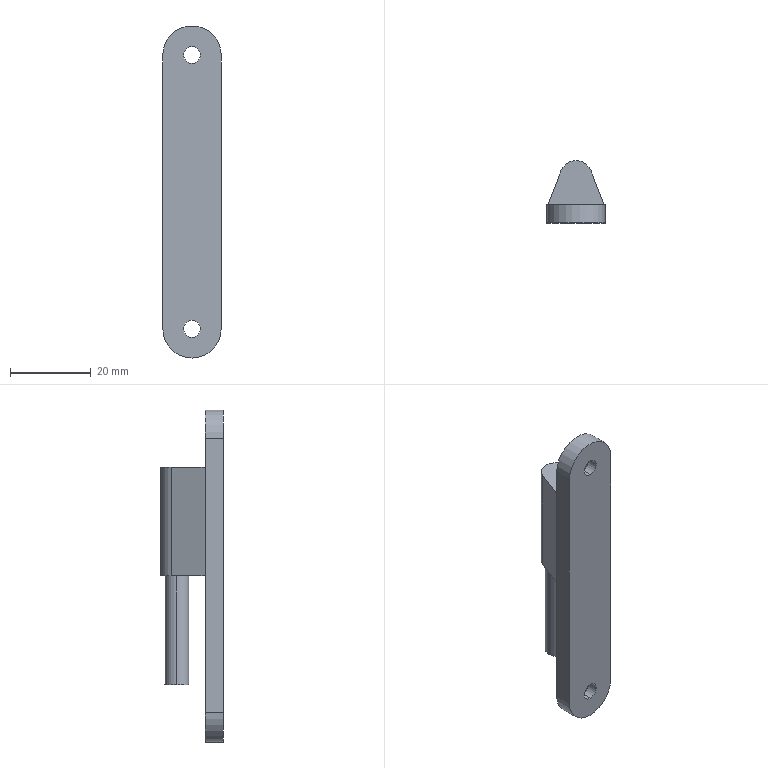Part | SolidWorks | features BaseBody 1 | 1 solid | 23 faces | box 14.5 x 15.5 x 82.5 mm | volume 8558 mm3 | cylinder 10 | plane 9 | cone 4 | commonest cylinder face diameters 4.2 x4 14.5 x3 6 x2 8 x1
STEP:
#1=CARTESIAN_POINT('',(-7.25,-7.,-34.));
#2=VERTEX_POINT('',#1);
#3=CARTESIAN_POINT('',(0.,-7.,-41.25));
#4=VERTEX_POINT('',#3);
#5=CARTESIAN_POINT('',(0.,-7.,-34.));
#6=DIRECTION('',(0.,-1.,0.));
#7=DIRECTION('',(0.,0.,-1.));
#8=AXIS2_PLACEMENT_3D('',#5,#6,#7);
#9=CIRCLE('',#8,7.25);
#10=EDGE_CURVE('',#2,#4,#9,.T.);
#11=ORIENTED_EDGE('',*,*,#10,.T.);
#12=CARTESIAN_POINT('',(0.,-11.5,-41.25));
#13=VERTEX_POINT('',#12);
#14=CARTESIAN_POINT('',(0.,-11.5,-41.25));
#15=DIRECTION('',(0.,-1.,0.));
#16=VECTOR('',#15,1000.);
#17=LINE('',#14,#16);
#18=EDGE_CURVE('',#4,#13,#17,.T.);
#19=ORIENTED_EDGE('',*,*,#18,.T.);
#20=CARTESIAN_POINT('',(-7.25,-11.5,-34.));
#21=VERTEX_POINT('',#20);
#22=CARTESIAN_POINT('',(0.,-11.5,-34.));
#23=DIRECTION('',(0.,1.,0.));
#24=DIRECTION('',(0.,0.,-1.));
#25=AXIS2_PLACEMENT_3D('',#22,#23,#24);
#26=CIRCLE('',#25,7.25);
#27=EDGE_CURVE('',#13,#21,#26,.T.);
#28=ORIENTED_EDGE('',*,*,#27,.T.);
#29=CARTESIAN_POINT('',(-7.25,-11.5,-34.));
#30=DIRECTION('',(0.,-1.,0.));
#31=VECTOR('',#30,1000.);
#32=LINE('',#29,#31);
#33=EDGE_CURVE('',#2,#21,#32,.T.);
#34=ORIENTED_EDGE('',*,*,#33,.F.);
#35=EDGE_LOOP('',(#11,#19,#28,#34));
#36=FACE_OUTER_BOUND('',#35,.T.);
#37=CARTESIAN_POINT('',(0.,-11.5,-34.));
#38=DIRECTION('',(0.,-1.,0.));
#39=DIRECTION('',(0.,0.,-1.));
#40=AXIS2_PLACEMENT_3D('',#37,#38,#39);
#41=CYLINDRICAL_SURFACE('',#40,7.25);
#42=ADVANCED_FACE('',(#36),#41,.T.);
#43=CARTESIAN_POINT('',(0.,-9.,36.1));
#44=VERTEX_POINT('',#43);
#45=CARTESIAN_POINT('',(0.,-9.,31.9));
#46=VERTEX_POINT('',#45);
#47=CARTESIAN_POINT('',(0.,-9.,34.));
#48=DIRECTION('',(0.,-1.,0.));
#49=DIRECTION('',(0.,0.,-1.));
#50=AXIS2_PLACEMENT_3D('',#47,#48,#49);
#51=CIRCLE('',#50,2.1);
#52=EDGE_CURVE('',#44,#46,#51,.T.);
#53=ORIENTED_EDGE('',*,*,#52,.F.);
#54=CARTESIAN_POINT('',(0.,-11.5,36.1));
#55=VERTEX_POINT('',#54);
#56=CARTESIAN_POINT('',(0.,-11.5,36.1));
#57=DIRECTION('',(0.,-1.,0.));
#58=VECTOR('',#57,1000.);
#59=LINE('',#56,#58);
#60=EDGE_CURVE('',#44,#55,#59,.T.);
#61=ORIENTED_EDGE('',*,*,#60,.T.);
#62=CARTESIAN_POINT('',(0.,-11.5,31.9));
#63=VERTEX_POINT('',#62);
#64=CARTESIAN_POINT('',(0.,-11.5,34.));
#65=DIRECTION('',(0.,-1.,0.));
#66=DIRECTION('',(0.,0.,-1.));
#67=AXIS2_PLACEMENT_3D('',#64,#65,#66);
#68=CIRCLE('',#67,2.1);
#69=EDGE_CURVE('',#55,#63,#68,.T.);
#70=ORIENTED_EDGE('',*,*,#69,.T.);
#71=CARTESIAN_POINT('',(0.,-11.5,31.9));
#72=DIRECTION('',(0.,-1.,0.));
#73=VECTOR('',#72,1000.);
#74=LINE('',#71,#73);
#75=EDGE_CURVE('',#46,#63,#74,.T.);
#76=ORIENTED_EDGE('',*,*,#75,.F.);
#77=EDGE_LOOP('',(#53,#61,#70,#76));
#78=FACE_OUTER_BOUND('',#77,.T.);
#79=CARTESIAN_POINT('',(0.,-11.5,34.));
#80=DIRECTION('',(0.,-1.,0.));
#81=DIRECTION('',(0.,0.,-1.));
#82=AXIS2_PLACEMENT_3D('',#79,#80,#81);
#83=CYLINDRICAL_SURFACE('',#82,2.1);
#84=ADVANCED_FACE('',(#78),#83,.F.);
#85=CARTESIAN_POINT('',(0.,-9.,-31.9));
#86=VERTEX_POINT('',#85);
#87=CARTESIAN_POINT('',(0.,-9.,-36.1));
#88=VERTEX_POINT('',#87);
#89=CARTESIAN_POINT('',(0.,-9.,-34.));
#90=DIRECTION('',(0.,-1.,0.));
#91=DIRECTION('',(0.,0.,-1.));
#92=AXIS2_PLACEMENT_3D('',#89,#90,#91);
#93=CIRCLE('',#92,2.1);
#94=EDGE_CURVE('',#86,#88,#93,.T.);
#95=ORIENTED_EDGE('',*,*,#94,.F.);
#96=CARTESIAN_POINT('',(0.,-11.5,-31.9));
#97=VERTEX_POINT('',#96);
#98=CARTESIAN_POINT('',(0.,-11.5,-31.9));
#99=DIRECTION('',(0.,-1.,0.));
#100=VECTOR('',#99,1000.);
#101=LINE('',#98,#100);
#102=EDGE_CURVE('',#86,#97,#101,.T.);
#103=ORIENTED_EDGE('',*,*,#102,.T.);
#104=CARTESIAN_POINT('',(0.,-11.5,-36.1));
#105=VERTEX_POINT('',#104);
#106=CARTESIAN_POINT('',(0.,-11.5,-34.));
#107=DIRECTION('',(0.,-1.,0.));
#108=DIRECTION('',(0.,0.,-1.));
#109=AXIS2_PLACEMENT_3D('',#106,#107,#108);
#110=CIRCLE('',#109,2.1);
#111=EDGE_CURVE('',#97,#105,#110,.T.);
#112=ORIENTED_EDGE('',*,*,#111,.T.);
#113=CARTESIAN_POINT('',(0.,-11.5,-36.1));
#114=DIRECTION('',(0.,-1.,0.));
#115=VECTOR('',#114,1000.);
#116=LINE('',#113,#115);
#117=EDGE_CURVE('',#88,#105,#116,.T.);
#118=ORIENTED_EDGE('',*,*,#117,.F.);
#119=EDGE_LOOP('',(#95,#103,#112,#118));
#120=FACE_OUTER_BOUND('',#119,.T.);
#121=CARTESIAN_POINT('',(0.,-11.5,-34.));
#122=DIRECTION('',(0.,-1.,0.));
#123=DIRECTION('',(0.,0.,-1.));
#124=AXIS2_PLACEMENT_3D('',#121,#122,#123);
#125=CYLINDRICAL_SURFACE('',#124,2.1);
#126=ADVANCED_FACE('',(#120),#125,.F.);
#127=ORIENTED_EDGE('',*,*,#52,.T.);
#128=CARTESIAN_POINT('',(0.,-7.,29.9));
#129=VERTEX_POINT('',#128);
#130=CARTESIAN_POINT('',(0.,-7.,29.9));
#131=DIRECTION('',(0.,0.7071,-0.7071));
#132=VECTOR('',#131,1000.);
#133=LINE('',#130,#132);
#134=EDGE_CURVE('',#46,#129,#133,.T.);
#135=ORIENTED_EDGE('',*,*,#134,.T.);
#136=CARTESIAN_POINT('',(0.,-7.,38.1));
#137=VERTEX_POINT('',#136);
#138=CARTESIAN_POINT('',(0.,-7.,34.));
#139=DIRECTION('',(0.,-1.,0.));
#140=DIRECTION('',(0.,0.,1.));
#141=AXIS2_PLACEMENT_3D('',#138,#139,#140);
#142=CIRCLE('',#141,4.1);
#143=EDGE_CURVE('',#137,#129,#142,.T.);
#144=ORIENTED_EDGE('',*,*,#143,.F.);
#145=CARTESIAN_POINT('',(0.,-7.,38.1));
#146=DIRECTION('',(0.,0.7071,0.7071));
#147=VECTOR('',#146,1000.);
#148=LINE('',#145,#147);
#149=EDGE_CURVE('',#44,#137,#148,.T.);
#150=ORIENTED_EDGE('',*,*,#149,.F.);
#151=EDGE_LOOP('',(#127,#135,#144,#150));
#152=FACE_OUTER_BOUND('',#151,.T.);
#153=CARTESIAN_POINT('',(0.,-7.,34.));
#154=DIRECTION('',(0.,1.,0.));
#155=DIRECTION('',(0.,0.,1.));
#156=AXIS2_PLACEMENT_3D('',#153,#154,#155);
#157=CONICAL_SURFACE('',#156,4.1,0.7854);
#158=ADVANCED_FACE('',(#152),#157,.F.);
#159=ORIENTED_EDGE('',*,*,#94,.T.);
#160=CARTESIAN_POINT('',(0.,-7.,-38.1));
#161=VERTEX_POINT('',#160);
#162=CARTESIAN_POINT('',(0.,-7.,-38.1));
#163=DIRECTION('',(0.,0.7071,-0.7071));
#164=VECTOR('',#163,1000.);
#165=LINE('',#162,#164);
#166=EDGE_CURVE('',#88,#161,#165,.T.);
#167=ORIENTED_EDGE('',*,*,#166,.T.);
#168=CARTESIAN_POINT('',(0.,-7.,-29.9));
#169=VERTEX_POINT('',#168);
#170=CARTESIAN_POINT('',(0.,-7.,-34.));
#171=DIRECTION('',(0.,-1.,0.));
#172=DIRECTION('',(0.,0.,1.));
#173=AXIS2_PLACEMENT_3D('',#170,#171,#172);
#174=CIRCLE('',#173,4.1);
#175=EDGE_CURVE('',#169,#161,#174,.T.);
#176=ORIENTED_EDGE('',*,*,#175,.F.);
#177=CARTESIAN_POINT('',(0.,-7.,-29.9));
#178=DIRECTION('',(0.,0.7071,0.7071));
#179=VECTOR('',#178,1000.);
#180=LINE('',#177,#179);
#181=EDGE_CURVE('',#86,#169,#180,.T.);
#182=ORIENTED_EDGE('',*,*,#181,.F.);
#183=EDGE_LOOP('',(#159,#167,#176,#182));
#184=FACE_OUTER_BOUND('',#183,.T.);
#185=CARTESIAN_POINT('',(0.,-7.,-34.));
#186=DIRECTION('',(0.,1.,0.));
#187=DIRECTION('',(0.,0.,1.));
#188=AXIS2_PLACEMENT_3D('',#185,#186,#187);
#189=CONICAL_SURFACE('',#188,4.1,0.7854);
#190=ADVANCED_FACE('',(#184),#189,.F.);
#191=CARTESIAN_POINT('',(3.,0.,-27.));
#192=VERTEX_POINT('',#191);
#193=CARTESIAN_POINT('',(-3.,0.,-27.));
#194=VERTEX_POINT('',#193);
#195=CARTESIAN_POINT('',(0.,0.,-27.));
#196=DIRECTION('',(0.,0.,1.));
#197=DIRECTION('',(1.,0.,0.));
#198=AXIS2_PLACEMENT_3D('',#195,#196,#197);
#199=CIRCLE('',#198,3.);
#200=EDGE_CURVE('',#192,#194,#199,.T.);
#201=ORIENTED_EDGE('',*,*,#200,.T.);
#202=CARTESIAN_POINT('',(-3.,0.,0.));
#203=VERTEX_POINT('',#202);
#204=CARTESIAN_POINT('',(-3.,0.,27.));
#205=DIRECTION('',(0.,0.,1.));
#206=VECTOR('',#205,1000.);
#207=LINE('',#204,#206);
#208=EDGE_CURVE('',#194,#203,#207,.T.);
#209=ORIENTED_EDGE('',*,*,#208,.T.);
#210=CARTESIAN_POINT('',(3.,0.,0.));
#211=VERTEX_POINT('',#210);
#212=CARTESIAN_POINT('',(0.,0.,0.));
#213=DIRECTION('',(0.,0.,-1.));
#214=DIRECTION('',(1.,0.,0.));
#215=AXIS2_PLACEMENT_3D('',#212,#213,#214);
#216=CIRCLE('',#215,3.);
#217=EDGE_CURVE('',#203,#211,#216,.T.);
#218=ORIENTED_EDGE('',*,*,#217,.T.);
#219=CARTESIAN_POINT('',(3.,0.,27.));
#220=DIRECTION('',(0.,0.,1.));
#221=VECTOR('',#220,1000.);
#222=LINE('',#219,#221);
#223=EDGE_CURVE('',#192,#211,#222,.T.);
#224=ORIENTED_EDGE('',*,*,#223,.F.);
#225=EDGE_LOOP('',(#201,#209,#218,#224));
#226=FACE_OUTER_BOUND('',#225,.T.);
#227=CARTESIAN_POINT('',(0.,0.,27.));
#228=DIRECTION('',(0.,0.,1.));
#229=DIRECTION('',(1.,0.,0.));
#230=AXIS2_PLACEMENT_3D('',#227,#228,#229);
#231=CYLINDRICAL_SURFACE('',#230,3.);
#232=ADVANCED_FACE('',(#226),#231,.T.);
#233=CARTESIAN_POINT('',(7.25,-11.5,-34.));
#234=VERTEX_POINT('',#233);
#235=CARTESIAN_POINT('',(0.,-11.5,-34.));
#236=DIRECTION('',(0.,1.,0.));
#237=DIRECTION('',(0.,0.,-1.));
#238=AXIS2_PLACEMENT_3D('',#235,#236,#237);
#239=CIRCLE('',#238,7.25);
#240=EDGE_CURVE('',#234,#13,#239,.T.);
#241=ORIENTED_EDGE('',*,*,#240,.F.);
#242=CARTESIAN_POINT('',(7.25,-11.5,34.));
#243=VERTEX_POINT('',#242);
#244=CARTESIAN_POINT('',(7.25,-11.5,34.));
#245=DIRECTION('',(0.,0.,-1.));
#246=VECTOR('',#245,1000.);
#247=LINE('',#244,#246);
#248=EDGE_CURVE('',#243,#234,#247,.T.);
#249=ORIENTED_EDGE('',*,*,#248,.F.);
#250=CARTESIAN_POINT('',(-7.25,-11.5,34.));
#251=VERTEX_POINT('',#250);
#252=CARTESIAN_POINT('',(0.,-11.5,34.));
#253=DIRECTION('',(0.,1.,0.));
#254=DIRECTION('',(0.,0.,-1.));
#255=AXIS2_PLACEMENT_3D('',#252,#253,#254);
#256=CIRCLE('',#255,7.25);
#257=EDGE_CURVE('',#251,#243,#256,.T.);
#258=ORIENTED_EDGE('',*,*,#257,.F.);
#259=CARTESIAN_POINT('',(-7.25,-11.5,34.));
#260=DIRECTION('',(0.,0.,1.));
#261=VECTOR('',#260,1000.);
#262=LINE('',#259,#261);
#263=EDGE_CURVE('',#21,#251,#262,.T.);
#264=ORIENTED_EDGE('',*,*,#263,.F.);
#265=ORIENTED_EDGE('',*,*,#27,.F.);
#266=EDGE_LOOP('',(#241,#249,#258,#264,#265));
#267=FACE_OUTER_BOUND('',#266,.T.);
#268=CARTESIAN_POINT('',(0.,-11.5,34.));
#269=DIRECTION('',(0.,-1.,0.));
#270=DIRECTION('',(0.,0.,-1.));
#271=AXIS2_PLACEMENT_3D('',#268,#269,#270);
#272=CIRCLE('',#271,2.1);
#273=EDGE_CURVE('',#63,#55,#272,.T.);
#274=ORIENTED_EDGE('',*,*,#273,.F.);
#275=ORIENTED_EDGE('',*,*,#69,.F.);
#276=EDGE_LOOP('',(#274,#275));
#277=FACE_BOUND('',#276,.T.);
#278=CARTESIAN_POINT('',(0.,-11.5,-34.));
#279=DIRECTION('',(0.,-1.,0.));
#280=DIRECTION('',(0.,0.,-1.));
#281=AXIS2_PLACEMENT_3D('',#278,#279,#280);
#282=CIRCLE('',#281,2.1);
#283=EDGE_CURVE('',#105,#97,#282,.T.);
#284=ORIENTED_EDGE('',*,*,#283,.F.);
#285=ORIENTED_EDGE('',*,*,#111,.F.);
#286=EDGE_LOOP('',(#284,#285));
#287=FACE_BOUND('',#286,.T.);
#288=CARTESIAN_POINT('',(0.,-11.5,34.));
#289=DIRECTION('',(0.,1.,0.));
#290=DIRECTION('',(0.,0.,1.));
#291=AXIS2_PLACEMENT_3D('',#288,#289,#290);
#292=PLANE('',#291);
#293=ADVANCED_FACE('',(#267,#277,#287),#292,.F.);
#294=ORIENTED_EDGE('',*,*,#263,.T.);
#295=CARTESIAN_POINT('',(-7.25,-7.,34.));
#296=VERTEX_POINT('',#295);
#297=CARTESIAN_POINT('',(-7.25,-11.5,34.));
#298=DIRECTION('',(0.,1.,0.));
#299=VECTOR('',#298,1000.);
#300=LINE('',#297,#299);
#301=EDGE_CURVE('',#251,#296,#300,.T.);
#302=ORIENTED_EDGE('',*,*,#301,.T.);
#303=CARTESIAN_POINT('',(-7.25,-7.,-34.));
#304=DIRECTION('',(0.,0.,-1.));
#305=VECTOR('',#304,1000.);
#306=LINE('',#303,#305);
#307=EDGE_CURVE('',#296,#2,#306,.T.);
#308=ORIENTED_EDGE('',*,*,#307,.T.);
#309=ORIENTED_EDGE('',*,*,#33,.T.);
#310=EDGE_LOOP('',(#294,#302,#308,#309));
#311=FACE_OUTER_BOUND('',#310,.T.);
#312=CARTESIAN_POINT('',(-7.25,-11.5,-34.));
#313=DIRECTION('',(-1.,0.,0.));
#314=DIRECTION('',(0.,0.,1.));
#315=AXIS2_PLACEMENT_3D('',#312,#313,#314);
#316=PLANE('',#315);
#317=ADVANCED_FACE('',(#311),#316,.T.);
#318=ORIENTED_EDGE('',*,*,#18,.F.);
#319=CARTESIAN_POINT('',(7.25,-7.,-34.));
#320=VERTEX_POINT('',#319);
#321=CARTESIAN_POINT('',(0.,-7.,-34.));
#322=DIRECTION('',(0.,-1.,0.));
#323=DIRECTION('',(0.,0.,-1.));
#324=AXIS2_PLACEMENT_3D('',#321,#322,#323);
#325=CIRCLE('',#324,7.25);
#326=EDGE_CURVE('',#4,#320,#325,.T.);
#327=ORIENTED_EDGE('',*,*,#326,.T.);
#328=CARTESIAN_POINT('',(7.25,-11.5,-34.));
#329=DIRECTION('',(0.,-1.,0.));
#330=VECTOR('',#329,1000.);
#331=LINE('',#328,#330);
#332=EDGE_CURVE('',#320,#234,#331,.T.);
#333=ORIENTED_EDGE('',*,*,#332,.T.);
#334=ORIENTED_EDGE('',*,*,#240,.T.);
#335=EDGE_LOOP('',(#318,#327,#333,#334));
#336=FACE_OUTER_BOUND('',#335,.T.);
#337=CARTESIAN_POINT('',(0.,-11.5,-34.));
#338=DIRECTION('',(0.,-1.,0.));
#339=DIRECTION('',(0.,0.,-1.));
#340=AXIS2_PLACEMENT_3D('',#337,#338,#339);
#341=CYLINDRICAL_SURFACE('',#340,7.25);
#342=ADVANCED_FACE('',(#336),#341,.T.);
#343=ORIENTED_EDGE('',*,*,#248,.T.);
#344=ORIENTED_EDGE('',*,*,#332,.F.);
#345=CARTESIAN_POINT('',(7.25,-7.,34.));
#346=VERTEX_POINT('',#345);
#347=CARTESIAN_POINT('',(7.25,-7.,34.));
#348=DIRECTION('',(0.,0.,1.));
#349=VECTOR('',#348,1000.);
#350=LINE('',#347,#349);
#351=EDGE_CURVE('',#320,#346,#350,.T.);
#352=ORIENTED_EDGE('',*,*,#351,.T.);
#353=CARTESIAN_POINT('',(7.25,-11.5,34.));
#354=DIRECTION('',(0.,-1.,0.));
#355=VECTOR('',#354,1000.);
#356=LINE('',#353,#355);
#357=EDGE_CURVE('',#346,#243,#356,.T.);
#358=ORIENTED_EDGE('',*,*,#357,.T.);
#359=EDGE_LOOP('',(#343,#344,#352,#358));
#360=FACE_OUTER_BOUND('',#359,.T.);
#361=CARTESIAN_POINT('',(7.25,-11.5,34.));
#362=DIRECTION('',(1.,0.,0.));
#363=DIRECTION('',(0.,0.,-1.));
#364=AXIS2_PLACEMENT_3D('',#361,#362,#363);
#365=PLANE('',#364);
#366=ADVANCED_FACE('',(#360),#365,.T.);
#367=ORIENTED_EDGE('',*,*,#257,.T.);
#368=ORIENTED_EDGE('',*,*,#357,.F.);
#369=CARTESIAN_POINT('',(0.,-7.,34.));
#370=DIRECTION('',(0.,-1.,0.));
#371=DIRECTION('',(0.,0.,-1.));
#372=AXIS2_PLACEMENT_3D('',#369,#370,#371);
#373=CIRCLE('',#372,7.25);
#374=EDGE_CURVE('',#346,#296,#373,.T.);
#375=ORIENTED_EDGE('',*,*,#374,.T.);
#376=ORIENTED_EDGE('',*,*,#301,.F.);
#377=EDGE_LOOP('',(#367,#368,#375,#376));
#378=FACE_OUTER_BOUND('',#377,.T.);
#379=CARTESIAN_POINT('',(0.,-11.5,34.));
#380=DIRECTION('',(0.,-1.,0.));
#381=DIRECTION('',(0.,0.,-1.));
#382=AXIS2_PLACEMENT_3D('',#379,#380,#381);
#383=CYLINDRICAL_SURFACE('',#382,7.25);
#384=ADVANCED_FACE('',(#378),#383,.T.);
#385=ORIENTED_EDGE('',*,*,#60,.F.);
#386=CARTESIAN_POINT('',(0.,-9.,34.));
#387=DIRECTION('',(0.,-1.,0.));
#388=DIRECTION('',(0.,0.,-1.));
#389=AXIS2_PLACEMENT_3D('',#386,#387,#388);
#390=CIRCLE('',#389,2.1);
#391=EDGE_CURVE('',#46,#44,#390,.T.);
#392=ORIENTED_EDGE('',*,*,#391,.F.);
#393=ORIENTED_EDGE('',*,*,#75,.T.);
#394=ORIENTED_EDGE('',*,*,#273,.T.);
#395=EDGE_LOOP('',(#385,#392,#393,#394));
#396=FACE_OUTER_BOUND('',#395,.T.);
#397=CARTESIAN_POINT('',(0.,-11.5,34.));
#398=DIRECTION('',(0.,-1.,0.));
#399=DIRECTION('',(0.,0.,-1.));
#400=AXIS2_PLACEMENT_3D('',#397,#398,#399);
#401=CYLINDRICAL_SURFACE('',#400,2.1);
#402=ADVANCED_FACE('',(#396),#401,.F.);
#403=ORIENTED_EDGE('',*,*,#102,.F.);
#404=CARTESIAN_POINT('',(0.,-9.,-34.));
#405=DIRECTION('',(0.,-1.,0.));
#406=DIRECTION('',(0.,0.,-1.));
#407=AXIS2_PLACEMENT_3D('',#404,#405,#406);
#408=CIRCLE('',#407,2.1);
#409=EDGE_CURVE('',#88,#86,#408,.T.);
#410=ORIENTED_EDGE('',*,*,#409,.F.);
#411=ORIENTED_EDGE('',*,*,#117,.T.);
#412=ORIENTED_EDGE('',*,*,#283,.T.);
#413=EDGE_LOOP('',(#403,#410,#411,#412));
#414=FACE_OUTER_BOUND('',#413,.T.);
#415=CARTESIAN_POINT('',(0.,-11.5,-34.));
#416=DIRECTION('',(0.,-1.,0.));
#417=DIRECTION('',(0.,0.,-1.));
#418=AXIS2_PLACEMENT_3D('',#415,#416,#417);
#419=CYLINDRICAL_SURFACE('',#418,2.1);
#420=ADVANCED_FACE('',(#414),#419,.F.);
#421=ORIENTED_EDGE('',*,*,#175,.T.);
#422=CARTESIAN_POINT('',(0.,-7.,-34.));
#423=DIRECTION('',(0.,-1.,0.));
#424=DIRECTION('',(0.,0.,1.));
#425=AXIS2_PLACEMENT_3D('',#422,#423,#424);
#426=CIRCLE('',#425,4.1);
#427=EDGE_CURVE('',#161,#169,#426,.T.);
#428=ORIENTED_EDGE('',*,*,#427,.T.);
#429=EDGE_LOOP('',(#421,#428));
#430=FACE_BOUND('',#429,.T.);
#431=ORIENTED_EDGE('',*,*,#351,.F.);
#432=ORIENTED_EDGE('',*,*,#326,.F.);
#433=ORIENTED_EDGE('',*,*,#10,.F.);
#434=ORIENTED_EDGE('',*,*,#307,.F.);
#435=ORIENTED_EDGE('',*,*,#374,.F.);
#436=EDGE_LOOP('',(#431,#432,#433,#434,#435));
#437=FACE_OUTER_BOUND('',#436,.T.);
#438=CARTESIAN_POINT('',(-6.95,-7.,27.));
#439=VERTEX_POINT('',#438);
#440=CARTESIAN_POINT('',(-6.95,-7.,0.));
#441=VERTEX_POINT('',#440);
#442=CARTESIAN_POINT('',(-6.95,-7.,34.));
#443=DIRECTION('',(0.,0.,-1.));
#444=VECTOR('',#443,1000.);
#445=LINE('',#442,#444);
#446=EDGE_CURVE('',#439,#441,#445,.T.);
#447=ORIENTED_EDGE('',*,*,#446,.T.);
#448=CARTESIAN_POINT('',(6.95,-7.,0.));
#449=VERTEX_POINT('',#448);
#450=CARTESIAN_POINT('',(0.,-7.,0.));
#451=DIRECTION('',(1.,0.,0.));
#452=VECTOR('',#451,1000.);
#453=LINE('',#450,#452);
#454=EDGE_CURVE('',#441,#449,#453,.T.);
#455=ORIENTED_EDGE('',*,*,#454,.T.);
#456=CARTESIAN_POINT('',(6.95,-7.,27.));
#457=VERTEX_POINT('',#456);
#458=CARTESIAN_POINT('',(6.95,-7.,34.));
#459=DIRECTION('',(0.,0.,1.));
#460=VECTOR('',#459,1000.);
#461=LINE('',#458,#460);
#462=EDGE_CURVE('',#449,#457,#461,.T.);
#463=ORIENTED_EDGE('',*,*,#462,.T.);
#464=CARTESIAN_POINT('',(0.,-7.,27.));
#465=DIRECTION('',(-1.,0.,0.));
#466=VECTOR('',#465,1000.);
#467=LINE('',#464,#466);
#468=EDGE_CURVE('',#457,#439,#467,.T.);
#469=ORIENTED_EDGE('',*,*,#468,.T.);
#470=EDGE_LOOP('',(#447,#455,#463,#469));
#471=FACE_BOUND('',#470,.T.);
#472=ORIENTED_EDGE('',*,*,#143,.T.);
#473=CARTESIAN_POINT('',(0.,-7.,34.));
#474=DIRECTION('',(0.,-1.,0.));
#475=DIRECTION('',(0.,0.,1.));
#476=AXIS2_PLACEMENT_3D('',#473,#474,#475);
#477=CIRCLE('',#476,4.1);
#478=EDGE_CURVE('',#129,#137,#477,.T.);
#479=ORIENTED_EDGE('',*,*,#478,.T.);
#480=EDGE_LOOP('',(#472,#479));
#481=FACE_BOUND('',#480,.T.);
#482=CARTESIAN_POINT('',(0.,-7.,34.));
#483=DIRECTION('',(0.,1.,0.));
#484=DIRECTION('',(0.,0.,1.));
#485=AXIS2_PLACEMENT_3D('',#482,#483,#484);
#486=PLANE('',#485);
#487=ADVANCED_FACE('',(#430,#437,#471,#481),#486,.T.);
#488=ORIENTED_EDGE('',*,*,#134,.F.);
#489=ORIENTED_EDGE('',*,*,#391,.T.);
#490=ORIENTED_EDGE('',*,*,#149,.T.);
#491=ORIENTED_EDGE('',*,*,#478,.F.);
#492=EDGE_LOOP('',(#488,#489,#490,#491));
#493=FACE_OUTER_BOUND('',#492,.T.);
#494=CARTESIAN_POINT('',(0.,-7.,34.));
#495=DIRECTION('',(0.,1.,0.));
#496=DIRECTION('',(0.,0.,1.));
#497=AXIS2_PLACEMENT_3D('',#494,#495,#496);
#498=CONICAL_SURFACE('',#497,4.1,0.7854);
#499=ADVANCED_FACE('',(#493),#498,.F.);
#500=ORIENTED_EDGE('',*,*,#166,.F.);
#501=ORIENTED_EDGE('',*,*,#409,.T.);
#502=ORIENTED_EDGE('',*,*,#181,.T.);
#503=ORIENTED_EDGE('',*,*,#427,.F.);
#504=EDGE_LOOP('',(#500,#501,#502,#503));
#505=FACE_OUTER_BOUND('',#504,.T.);
#506=CARTESIAN_POINT('',(0.,-7.,-34.));
#507=DIRECTION('',(0.,1.,0.));
#508=DIRECTION('',(0.,0.,1.));
#509=AXIS2_PLACEMENT_3D('',#506,#507,#508);
#510=CONICAL_SURFACE('',#509,4.1,0.7854);
#511=ADVANCED_FACE('',(#505),#510,.F.);
#512=CARTESIAN_POINT('',(3.738,1.425,0.));
#513=VERTEX_POINT('',#512);
#514=CARTESIAN_POINT('',(-3.738,1.425,0.));
#515=VERTEX_POINT('',#514);
#516=CARTESIAN_POINT('',(0.,0.,0.));
#517=DIRECTION('',(0.,0.,1.));
#518=DIRECTION('',(1.,0.,0.));
#519=AXIS2_PLACEMENT_3D('',#516,#517,#518);
#520=CIRCLE('',#519,4.);
#521=EDGE_CURVE('',#513,#515,#520,.T.);
#522=ORIENTED_EDGE('',*,*,#521,.F.);
#523=CARTESIAN_POINT('',(6.95,-7.,0.));
#524=DIRECTION('',(-0.3563,0.9344,0.));
#525=VECTOR('',#524,1000.);
#526=LINE('',#523,#525);
#527=EDGE_CURVE('',#449,#513,#526,.T.);
#528=ORIENTED_EDGE('',*,*,#527,.F.);
#529=ORIENTED_EDGE('',*,*,#454,.F.);
#530=CARTESIAN_POINT('',(-3.738,1.425,0.));
#531=DIRECTION('',(-0.3563,-0.9344,0.));
#532=VECTOR('',#531,1000.);
#533=LINE('',#530,#532);
#534=EDGE_CURVE('',#515,#441,#533,.T.);
#535=ORIENTED_EDGE('',*,*,#534,.F.);
#536=EDGE_LOOP('',(#522,#528,#529,#535));
#537=FACE_OUTER_BOUND('',#536,.T.);
#538=CARTESIAN_POINT('',(0.,0.,0.));
#539=DIRECTION('',(0.,0.,-1.));
#540=DIRECTION('',(1.,0.,0.));
#541=AXIS2_PLACEMENT_3D('',#538,#539,#540);
#542=CIRCLE('',#541,3.);
#543=EDGE_CURVE('',#211,#203,#542,.T.);
#544=ORIENTED_EDGE('',*,*,#543,.F.);
#545=ORIENTED_EDGE('',*,*,#217,.F.);
#546=EDGE_LOOP('',(#544,#545));
#547=FACE_BOUND('',#546,.T.);
#548=CARTESIAN_POINT('',(0.,0.,0.));
#549=DIRECTION('',(0.,0.,1.));
#550=DIRECTION('',(1.,0.,0.));
#551=AXIS2_PLACEMENT_3D('',#548,#549,#550);
#552=PLANE('',#551);
#553=ADVANCED_FACE('',(#537,#547),#552,.F.);
#554=ORIENTED_EDGE('',*,*,#446,.F.);
#555=CARTESIAN_POINT('',(-3.738,1.425,27.));
#556=VERTEX_POINT('',#555);
#557=CARTESIAN_POINT('',(-3.738,1.425,27.));
#558=DIRECTION('',(-0.3563,-0.9344,0.));
#559=VECTOR('',#558,1000.);
#560=LINE('',#557,#559);
#561=EDGE_CURVE('',#556,#439,#560,.T.);
#562=ORIENTED_EDGE('',*,*,#561,.F.);
#563=CARTESIAN_POINT('',(-3.738,1.425,27.));
#564=DIRECTION('',(0.,0.,1.));
#565=VECTOR('',#564,1000.);
#566=LINE('',#563,#565);
#567=EDGE_CURVE('',#515,#556,#566,.T.);
#568=ORIENTED_EDGE('',*,*,#567,.F.);
#569=ORIENTED_EDGE('',*,*,#534,.T.);
#570=EDGE_LOOP('',(#554,#562,#568,#569));
#571=FACE_OUTER_BOUND('',#570,.T.);
#572=CARTESIAN_POINT('',(-3.738,1.425,27.));
#573=DIRECTION('',(0.9344,-0.3563,0.));
#574=DIRECTION('',(0.3563,0.9344,0.));
#575=AXIS2_PLACEMENT_3D('',#572,#573,#574);
#576=PLANE('',#575);
#577=ADVANCED_FACE('',(#571),#576,.F.);
#578=CARTESIAN_POINT('',(3.738,1.425,27.));
#579=VERTEX_POINT('',#578);
#580=CARTESIAN_POINT('',(6.95,-7.,27.));
#581=DIRECTION('',(-0.3563,0.9344,0.));
#582=VECTOR('',#581,1000.);
#583=LINE('',#580,#582);
#584=EDGE_CURVE('',#457,#579,#583,.T.);
#585=ORIENTED_EDGE('',*,*,#584,.T.);
#586=CARTESIAN_POINT('',(0.,0.,27.));
#587=DIRECTION('',(0.,0.,1.));
#588=DIRECTION('',(1.,0.,0.));
#589=AXIS2_PLACEMENT_3D('',#586,#587,#588);
#590=CIRCLE('',#589,4.);
#591=EDGE_CURVE('',#579,#556,#590,.T.);
#592=ORIENTED_EDGE('',*,*,#591,.T.);
#593=ORIENTED_EDGE('',*,*,#561,.T.);
#594=ORIENTED_EDGE('',*,*,#468,.F.);
#595=EDGE_LOOP('',(#585,#592,#593,#594));
#596=FACE_OUTER_BOUND('',#595,.T.);
#597=CARTESIAN_POINT('',(0.,0.,27.));
#598=DIRECTION('',(0.,0.,1.));
#599=DIRECTION('',(1.,0.,0.));
#600=AXIS2_PLACEMENT_3D('',#597,#598,#599);
#601=PLANE('',#600);
#602=ADVANCED_FACE('',(#596),#601,.T.);
#603=CARTESIAN_POINT('',(3.738,1.425,27.));
#604=DIRECTION('',(0.,0.,-1.));
#605=VECTOR('',#604,1000.);
#606=LINE('',#603,#605);
#607=EDGE_CURVE('',#579,#513,#606,.T.);
#608=ORIENTED_EDGE('',*,*,#607,.F.);
#609=ORIENTED_EDGE('',*,*,#584,.F.);
#610=ORIENTED_EDGE('',*,*,#462,.F.);
#611=ORIENTED_EDGE('',*,*,#527,.T.);
#612=EDGE_LOOP('',(#608,#609,#610,#611));
#613=FACE_OUTER_BOUND('',#612,.T.);
#614=CARTESIAN_POINT('',(6.95,-7.,27.));
#615=DIRECTION('',(-0.9344,-0.3563,0.));
#616=DIRECTION('',(0.3563,-0.9344,0.));
#617=AXIS2_PLACEMENT_3D('',#614,#615,#616);
#618=PLANE('',#617);
#619=ADVANCED_FACE('',(#613),#618,.F.);
#620=ORIENTED_EDGE('',*,*,#591,.F.);
#621=ORIENTED_EDGE('',*,*,#607,.T.);
#622=ORIENTED_EDGE('',*,*,#521,.T.);
#623=ORIENTED_EDGE('',*,*,#567,.T.);
#624=EDGE_LOOP('',(#620,#621,#622,#623));
#625=FACE_OUTER_BOUND('',#624,.T.);
#626=CARTESIAN_POINT('',(0.,0.,27.));
#627=DIRECTION('',(0.,0.,1.));
#628=DIRECTION('',(1.,0.,0.));
#629=AXIS2_PLACEMENT_3D('',#626,#627,#628);
#630=CYLINDRICAL_SURFACE('',#629,4.);
#631=ADVANCED_FACE('',(#625),#630,.T.);
#632=ORIENTED_EDGE('',*,*,#208,.F.);
#633=CARTESIAN_POINT('',(0.,0.,-27.));
#634=DIRECTION('',(0.,0.,1.));
#635=DIRECTION('',(1.,0.,0.));
#636=AXIS2_PLACEMENT_3D('',#633,#634,#635);
#637=CIRCLE('',#636,3.);
#638=EDGE_CURVE('',#194,#192,#637,.T.);
#639=ORIENTED_EDGE('',*,*,#638,.T.);
#640=ORIENTED_EDGE('',*,*,#223,.T.);
#641=ORIENTED_EDGE('',*,*,#543,.T.);
#642=EDGE_LOOP('',(#632,#639,#640,#641));
#643=FACE_OUTER_BOUND('',#642,.T.);
#644=CARTESIAN_POINT('',(0.,0.,27.));
#645=DIRECTION('',(0.,0.,1.));
#646=DIRECTION('',(1.,0.,0.));
#647=AXIS2_PLACEMENT_3D('',#644,#645,#646);
#648=CYLINDRICAL_SURFACE('',#647,3.);
#649=ADVANCED_FACE('',(#643),#648,.T.);
#650=ORIENTED_EDGE('',*,*,#200,.F.);
#651=ORIENTED_EDGE('',*,*,#638,.F.);
#652=EDGE_LOOP('',(#650,#651));
#653=FACE_OUTER_BOUND('',#652,.T.);
#654=CARTESIAN_POINT('',(0.,0.,-27.));
#655=DIRECTION('',(0.,0.,1.));
#656=DIRECTION('',(1.,0.,0.));
#657=AXIS2_PLACEMENT_3D('',#654,#655,#656);
#658=PLANE('',#657);
#659=ADVANCED_FACE('',(#653),#658,.F.);
#660=CLOSED_SHELL('',(#42,#84,#126,#158,#190,#232,#293,#317,#342,#366,#384,#402,#420,#487,#499,#511,#553,#577,#602,#619,#631,#649,#659));
#661=MANIFOLD_SOLID_BREP('',#660);
#662=CARTESIAN_POINT('',(0.,0.,0.));
#663=DIRECTION('',(0.,0.,1.));
#664=DIRECTION('',(1.,0.,0.));
#665=AXIS2_PLACEMENT_3D('',#662,#663,#664);
#666=(LENGTH_UNIT()NAMED_UNIT(*)SI_UNIT(.MILLI.,.METRE.));
#667=UNCERTAINTY_MEASURE_WITH_UNIT(LENGTH_MEASURE(0.00001),#666,'','');
#668=(NAMED_UNIT(*)PLANE_ANGLE_UNIT()SI_UNIT($,.RADIAN.));
#669=(NAMED_UNIT(*)SI_UNIT($,.STERADIAN.)SOLID_ANGLE_UNIT());
#670=(GEOMETRIC_REPRESENTATION_CONTEXT(3)GLOBAL_UNCERTAINTY_ASSIGNED_CONTEXT((#667))GLOBAL_UNIT_ASSIGNED_CONTEXT((#666,#668,#669))REPRESENTATION_CONTEXT('',''));
#671=ADVANCED_BREP_SHAPE_REPRESENTATION('',(#661,#665),#670);